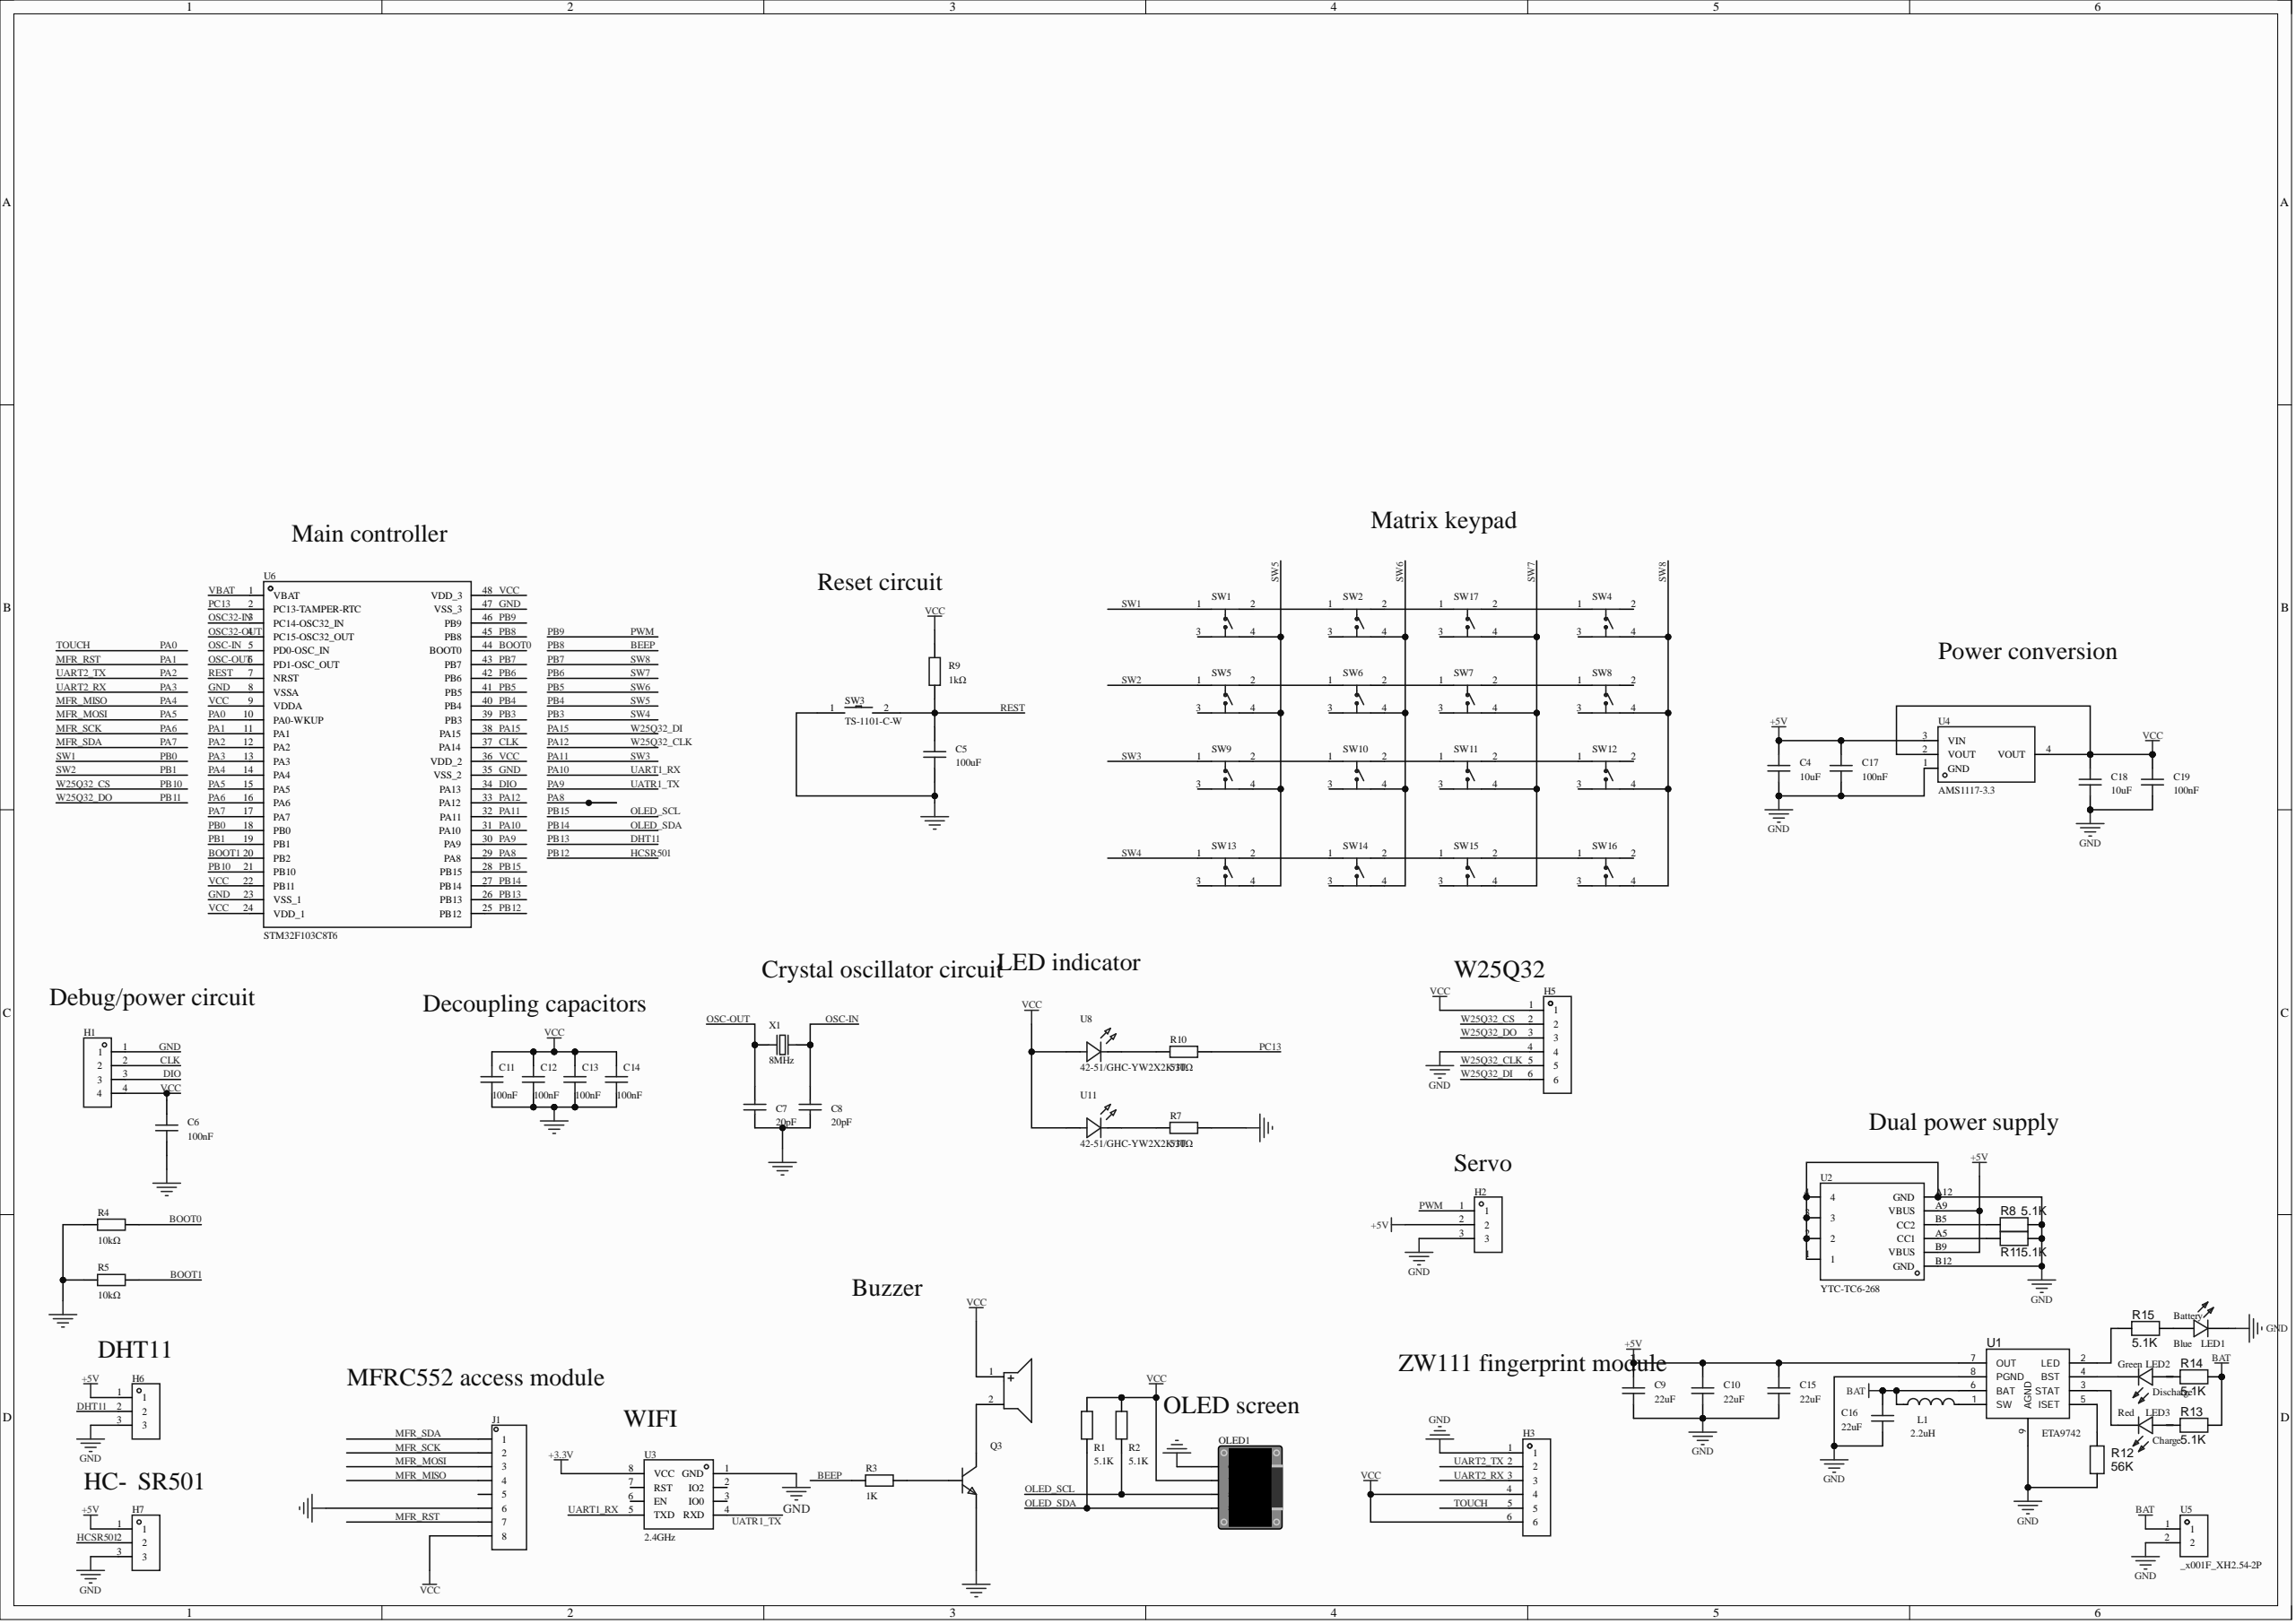Circuit board | Altium Designer | 70 parts | 65 nets
Bill of materials:
Comment,Description,Designator,Footprint,LibRef,Quantity
"2.7kHz","Drive: passive (external drive); construction: electromagnetic; frequency: 2.7kHz; sound pressure (SPL): 85dB;","BUZZER1","BUZ-TH_BD9.0-P4.00-D0.6-FD","QMB-09B-03","1"
"10uF","","C4, C18","C0603","CAP_0603","2"
"100uF","Capacitance: 100uF; tolerance: ±20%; rated voltage: 10V; dielectric (temperature coefficient): X5R;","C5","C1206","HGC1206R5107M100NSPJ","1"
"100nF","Capacitance: 100nF; tolerance: ±10%; rated voltage: 50V; dielectric (temperature coefficient): X7R;, [NoValue]","C6, C11, C12, C13, C14, C17, C19","C0603","CGA0603X7R104K500JT, CAP_0603","7"
"20pF","Capacitance: 20pF; tolerance: ±5%; rated voltage: 50V; dielectric (temperature coefficient): C0G;","C7, C8","C0603","CL10C200JB8NNNC","2"
"22uF","Capacitance: 22uF; tolerance: ±20%; rated voltage: 35V; dielectric (temperature coefficient): X5R;","C9, C10, C15, C16","C0603","C3216X5R1V226MTJ00E","4"
"","","H1","HDR-TH_4P-P2.54-V-F","HDR-F_2.54_1x4P","1"
"","","H2, H6, H7","HDR-TH_3P-P2.54-V-F","HDR-F_2.54_1x3P","3"
"","","H3, H5","HDR-TH_6P-P2.54-V-F","HDR-F_2.54_1x6P","2"
"","","J1","HDR-TH_8P-P2.54-V-M","HDR-M_2.54_1x8P","1"
"2.2uH","Inductance: 2.2uH; tolerance: ±20%; rated current: 4.5A; DC resistance (DCR): 58mΩ;","L1","IND-SMD_L4.4-W4.2","MWSA0402S-2R2MT","1"
"Battery","Emitted color: emerald green;","LED1","LED0603_L1.6-W0.8-RD_BLUE","NCD0603G1","1"
"Discharge","Emitted color: emerald green;","LED2","LED0603_L1.6-W0.8-RD_BLUE","NCD0603G1","1"
"Charge","Emitted color: emerald green;","LED3","LED0603_L1.6-W0.8-RD_BLUE","NCD0603G1","1"
"","","OLED1","0.96OLED_4P","0.96OLED模块_4P","1"
"","","Q3","S8050_TO_92","S8050_TO_NPN","1"
"5.1K","","R1, R2","R0603","Res_0603","2"
"1K","","R3","R0603","Res_0603","1"
"10kΩ","Resistor type: thick film resistor; resistance: 10kΩ; tolerance: ±1%; power: 100mW; max working voltage: 75V; temperature coefficient: ±100ppm/?;","R4, R5","R0603","0603WAF1002T5E","2"
"510Ω","Resistor type: thick film resistor; resistance: 510Ω; tolerance: ±1%; power: 100mW; max working voltage: 75V; temperature coefficient: ±100ppm/?;","R7, R10","R0603","0603WAF5100T5E","2"
"5.1K","","R8, R11, R13, R14, R15","R0603-NSK","NC","5"
"1kΩ","Resistor type: thick film resistor; resistance: 1kΩ; tolerance: ±1%; power: 100mW; max working voltage: 75V; temperature coefficient: ±100ppm/?;","R9","R0603","RC0603FR-071KL","1"
"56K","","R12","R0603-NSK","NC","1"
"KH-6X6X6H-TJ","","SW1, SW2, SW4, SW5, SW6, SW7, SW8, SW9, SW10, SW11, SW12, SW13, SW14, SW15, SW16, SW17","SW-TH_4P-L6.0-W6.0-P4.50-LS6.5","KH-6X6X6H-TJ","16"
"TS-1101-C-W","","SW3","SW-SMD_L6.0-W3.3-LS8.0","TS-1101-C-W","1"
"ETA9742","","U1","ESOP-8_L4.9-W3.9-P1.27-LS6.0-BL-EP","ETA9742","1"
"YTC-TC6-268","Connector type: Type-C; gender: female socket; contacts: 6;","U2","TYPE-C-SMD_YIYUAN_YTC-TC6-268","YTC-TC6-268","1"
"2.4GHz","Core processor: ESP8266 chip; frequency: 2.4GHz; antenna form: onboard PCB antenna; transmit power: 16dBm; receive sensitivity: -90dBm;","U3","WIFIM-TH_8P-L24.7-W14.4-P2.54","ESP-01S","1"
"AMS1117-3.3","Output type: fixed; working voltage: 15V; output voltage: 3.3V; output current: 1A; power supply rejection ratio (PSRR): 72dB@(120Hz); output polarity: positive;","U4","SOT-223-3_L6.5-W3.4-P2.30-LS7.0-BR","AMS1117-3.3_C6186","1"
"_x001F_XH2.54-2P","","U5","CONN-TH_2P-P2.54-V","_x001F_XH2.54-2P","1"
"STM32F103C8T6","","U6","LQFP-48_L7.0-W7.0-P0.50-LS9.0-BL","STM32F103C8T6","1"
"42-51/GHC-YW2X2K/3T","Emitted color: emerald green; forward current: -; dominant wavelength: 520nm~535nm; luminous intensity: 2850mcd;","U8, U11","LED-SMD_L1.6-W0.8-FD_GREEN-1","42-51/GHC-YW2X2K/3T","2"
"8MHz","Crystal type: SMD crystal; frequency: 8MHz; room-temperature frequency tolerance: ±10ppm; load capacitance: 12pF; frequency stability: ±20ppm;","X1","CRYSTAL-SMD_L3.2-W2.5_3225-8MHZ","X22EL89COI-111YLC-8M","1"
Netlist (Protel format):
[
BUZZER1
BUZ-TH_BD9.0-P4.00-D0.6-FD
2.7kHz



]
[
C4
C0603
10uF



]
[
C5
C1206
100uF



]
[
C6
C0603
100nF



]
[
C7
C0603
20pF



]
[
C8
C0603
20pF



]
[
C9
C0603
22uF



]
[
C10
C0603
22uF



]
[
C11
C0603
100nF



]
[
C12
C0603
100nF



]
[
C13
C0603
100nF



]
[
C14
C0603
100nF



]
[
C15
C0603
22uF



]
[
C16
C0603
22uF



]
[
C17
C0603
100nF



]
[
C18
C0603
10uF



]
[
C19
C0603
100nF



]
[
H1
HDR-TH_4P-P2.54-V-F




]
[
H2
HDR-TH_3P-P2.54-V-F




]
[
H3
HDR-TH_6P-P2.54-V-F




]
[
H5
HDR-TH_6P-P2.54-V-F




]
[
H6
HDR-TH_3P-P2.54-V-F




]
[
H7
HDR-TH_3P-P2.54-V-F




]
[
J1
HDR-TH_8P-P2.54-V-M




]
[
L1
IND-SMD_L4.4-W4.2
2.2uH



]
[
LED1
LED0603_L1.6-W0.8-RD_BLUE
Battery



]
[
LED2
LED0603_L1.6-W0.8-RD_BLUE
Discharge



]
[
LED3
LED0603_L1.6-W0.8-RD_BLUE
Charge



]
[
OLED1
0.96OLED_4P




]
[
Q3
S8050_TO_92




]
[
R1
R0603
5.1K



]
[
R2
R0603
5.1K



]
[
R3
R0603
1K



]
[
R4
R0603
10kΩ



]
[
R5
R0603
10kΩ



]
[
R7
R0603
510Ω



]
[
R8
R0603-NSK
5.1K



]
[
R9
R0603
1kΩ



]
[
R10
R0603
510Ω



]
[
R11
R0603-NSK
5.1K



]
[
R12
R0603-NSK
56K



]
[
R13
R0603-NSK
5.1K



]
[
R14
R0603-NSK
5.1K



]
[
R15
R0603-NSK
5.1K



]
[
SW1
SW-TH_4P-L6.0-W6.0-P4.50-LS6.5
KH-6X6X6H-TJ



]
[
SW2
SW-TH_4P-L6.0-W6.0-P4.50-LS6.5
KH-6X6X6H-TJ



]
[
SW3
SW-SMD_L6.0-W3.3-LS8.0
TS-1101-C-W



]
[
SW4
SW-TH_4P-L6.0-W6.0-P4.50-LS6.5
KH-6X6X6H-TJ



]
[
SW5
SW-TH_4P-L6.0-W6.0-P4.50-LS6.5
KH-6X6X6H-TJ



]
[
SW6
SW-TH_4P-L6.0-W6.0-P4.50-LS6.5
KH-6X6X6H-TJ



]
[
SW7
SW-TH_4P-L6.0-W6.0-P4.50-LS6.5
KH-6X6X6H-TJ



]
[
SW8
SW-TH_4P-L6.0-W6.0-P4.50-LS6.5
KH-6X6X6H-TJ



]
[
SW9
SW-TH_4P-L6.0-W6.0-P4.50-LS6.5
KH-6X6X6H-TJ



]
[
SW10
SW-TH_4P-L6.0-W6.0-P4.50-LS6.5
KH-6X6X6H-TJ



]
[
SW11
SW-TH_4P-L6.0-W6.0-P4.50-LS6.5
KH-6X6X6H-TJ



]
[
SW12
SW-TH_4P-L6.0-W6.0-P4.50-LS6.5
KH-6X6X6H-TJ



]
[
SW13
SW-TH_4P-L6.0-W6.0-P4.50-LS6.5
KH-6X6X6H-TJ



]
[
SW14
SW-TH_4P-L6.0-W6.0-P4.50-LS6.5
KH-6X6X6H-TJ



]
[
SW15
SW-TH_4P-L6.0-W6.0-P4.50-LS6.5
KH-6X6X6H-TJ



]
[
SW16
SW-TH_4P-L6.0-W6.0-P4.50-LS6.5
KH-6X6X6H-TJ



]
[
SW17
SW-TH_4P-L6.0-W6.0-P4.50-LS6.5
KH-6X6X6H-TJ



]
[
U1
ESOP-8_L4.9-W3.9-P1.27-LS6.0-BL-EP
ETA9742



]
[
U2
TYPE-C-SMD_YIYUAN_YTC-TC6-268
YTC-TC6-268



]
[
U3
WIFIM-TH_8P-L24.7-W14.4-P2.54
2.4GHz



]
[
U4
SOT-223-3_L6.5-W3.4-P2.30-LS7.0-BR
AMS1117-3.3



]
[
U5
CONN-TH_2P-P2.54-V
_x001F_XH2.54-2P



]
[
U6
LQFP-48_L7.0-W7.0-P0.50-LS9.0-BL
STM32F103C8T6



]
[
U8
LED-SMD_L1.6-W0.8-FD_GREEN-1
42-51/GHC-YW2X2K/3T



]
[
U11
LED-SMD_L1.6-W0.8-FD_GREEN-1
42-51/GHC-YW2X2K/3T



]
[
X1
CRYSTAL-SMD_L3.2-W2.5_3225-8MHZ
8MHz



]
(
VCC
BUZZER1-1
C6-2
C11-2
C12-2
C13-2
C14-2
C18-2
C19-2
H1-4
H3-4
H3-6
H5-1
J1-8
OLED1-2
R1-2
R2-2
R9-2
U4-2
U4-4
U6-9
U6-22
U6-24
U6-36
U6-48
U8-1
U11-1
)
(
REST
C5-2
R9-1
SW3-2
U6-7
)
(
PC13
R10-2
U6-2
)
(
PB10
H5-2
U6-21
)
(
PB9
H2-1
U6-46
)
(
PB7
SW4-4
SW8-4
SW12-4
SW16-4
U6-43
)
(
PB6
SW7-4
SW11-4
SW15-4
SW17-4
U6-42
)
(
PB5
SW2-4
SW6-4
SW10-4
SW14-4
U6-41
)
(
PB4
SW1-4
SW5-4
SW9-4
SW13-4
U6-40
)
(
PB3
SW13-1
U6-39
)
(
PB1
SW5-1
U6-19
)
(
PB0
SW1-1
U6-18
)
(
PA15
H5-6
U6-38
)
(
PA12
H5-5
U6-33
)
(
PA11
SW9-1
U6-32
)
(
PA10
U3-5
U6-31
)
(
PA9
U3-4
U6-30
)
(
PA3
H3-3
U6-13
)
(
PA2
H3-2
U6-12
)
(
PA0
H3-5
U6-10
)
(
OSC-OUT
C7-2
U6-6
X1-1
)
(
OSC-IN
C8-2
U6-5
X1-2
)
(
OLED_SDA
OLED1-4
R1-1
U6-27
)
(
OLED_SCL
OLED1-3
R2-1
U6-28
)
(
NetSW15_2
SW15-2
SW16-1
)
(
NetSW14_2
SW14-2
SW15-1
)
(
NetSW13_2
SW13-2
SW14-1
)
(
NetSW11_2
SW11-2
SW12-1
)
(
NetSW10_2
SW10-2
SW11-1
)
(
NetSW9_2
SW9-2
SW10-1
)
(
NetSW7_2
SW7-2
SW8-1
)
(
NetSW6_2
SW6-2
SW7-1
)
(
NetSW5_2
SW5-2
SW6-1
)
(
NetSW4_1
SW4-1
SW17-2
)
(
NetSW2_2
SW2-2
SW17-1
)
(
NetSW1_2
SW1-2
SW2-1
)
(
NetR15_2
R15-2
U1-2
)
(
NetR12_1
R12-1
U1-5
)
(
NetR11_2
R11-2
U2-A5
)
(
NetR10_1
R10-1
U8-2
)
(
NetR8_2
R8-2
U2-B5
)
(
NetR7_1
R7-1
U11-2
)
(
NetQ3_2
Q3-2
R3-1
)
(
NetLED3_2
LED3-2
R13-2
)
(
NetLED3_1
LED3-1
U1-3
)
(
NetLED2_2
LED2-2
R14-2
)
(
NetLED2_1
LED2-1
U1-4
)
(
NetLED1_2
LED1-2
R15-1
)
(
NetL1_2
L1-2
U1-1
)
(
NetBUZZER1_2
BUZZER1-2
Q3-3
)
(
MFR_SDA
J1-1
U6-17
)
(
MFR_SCK
J1-2
U6-16
)
(
MFR_RST
J1-7
U6-11
)
(
MFR_MOSI
J1-3
U6-15
)
(
MFR_MISO
J1-4
U6-14
)
(
HCSR501
H7-2
U6-25
)
(
GND
C4-1
C5-1
C6-1
C7-1
C8-1
C9-1
C10-1
C11-1
C12-1
C13-1
C14-1
C15-1
C16-1
C17-1
C18-1
C19-1
H1-1
H2-3
H3-1
H5-4
H6-3
H7-3
J1-6
LED1-1
OLED1-1
Q3-1
R4-1
R5-1
R7-2
R8-1
R11-1
R12-2
SW3-1
U1-8
U1-9
U2-1
U2-2
U2-3
U2-4
U2-A12
U2-B12
U3-1
U4-1
U5-2
U6-8
U6-23
U6-35
U6-47
)
(
DIO
H1-3
U6-34
)
(
DHT11
H6-2
U6-26
)
(
CLK
H1-2
U6-37
)
(
BOOT1
R5-2
U6-20
)
(
BOOT0
R4-2
U6-44
)
(
BEEP
R3-2
U6-45
)
(
BAT
C16-2
L1-1
R13-1
R14-1
U1-6
U5-1
)
(
+5V
C4-2
C9-2
C10-2
C15-2
C17-2
H2-2
H6-1
H7-1
U1-7
U2-A9
U2-B9
U4-3
)